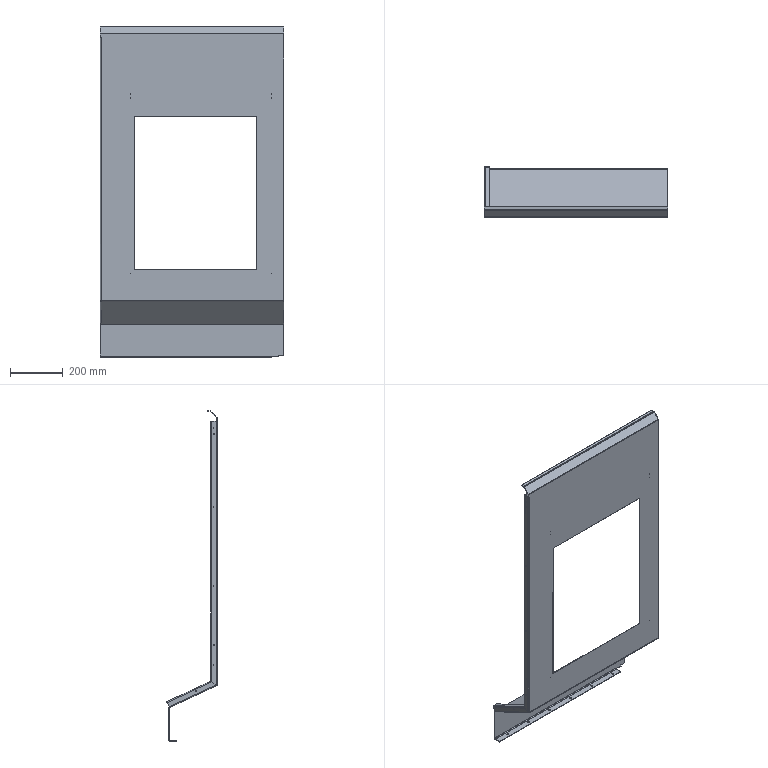Part | NX | features solid 2 | 1 solid | 112 faces | box 698 x 191.411 x 1253 mm | volume 1522478 mm3 | cylinder 56 | plane 52 | spline 4 | commonest cylinder face diameters 3.459 x14 1 x12 7 x12 4 x9 8 x9